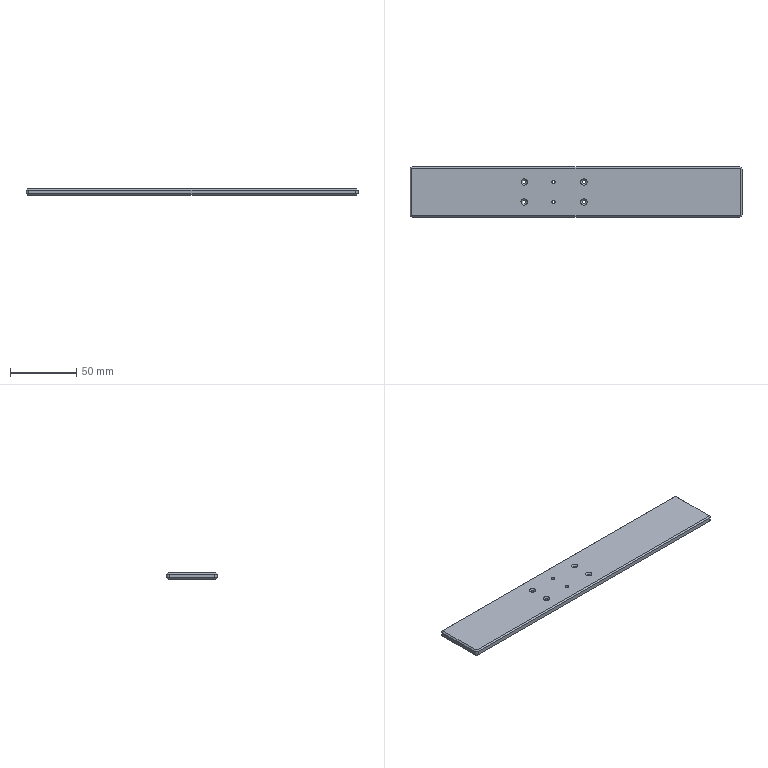CAM job | NX | 3-axis milling | part box 250 x 38 x 5 mm | stock box 256 x 44 x 5 mm
Tools:
number,name,description,diameter,corner_radius,flute_length,length,flutes
2,D10,Milling Tool-5 Parameters,10.0,0.0,50.0,75.0,2
8,D2,Milling Tool-5 Parameters,2.0,0.0,50.0,75.0,2
9,D6A45,Milling Tool-5 Parameters,6.0,0.0,3.0,3.0,2
6,D4,Milling Tool-5 Parameters,4.0,0.0,50.0,75.0,2
Operations:
program,operation,operation_type,tool,method,geometry_group,spindle_rpm,surface_speed,feed_per_tooth,feed_cut,feed_plunge,cut_length_mm,path_length_mm,cut_time_min,machine_time_min
PN_0001_BLANK_-_SUCTION_CUP,ZLEVEL_PROFILE,ZLevelMilling,D10,METHOD,A,6500.0,326.0,0.1538,2000.0,1000.0,3125.06,3186.76,1.586,1.592
PN_0001_BLANK_-_SUCTION_CUP,ZLEVEL_PROFILE_COPY_COPY_1_COPY_COPY_1_COPY,ZLevelMilling,D2,METHOD,A,7000.0,43.0,0.0714,1000.0,1000.0,1380.772,1838.533,1.381,1.427
PN_0001_BLANK_-_SUCTION_CUP,ZLEVEL_PROFILE_COPY_1_COPY_COPY_COPY_COPY_COPY_COPY,ZLevelMilling,D6A45,METHOD,A,7000.0,131.0,0.0714,1000.0,1000.0,582.053,646.053,0.5821,0.5885
PN_0001_BLANK_-_SUCTION_CUP,ZLEVEL_PROFILE_COPY_COPY_1_COPY,ZLevelMilling,D4,METHOD,A,6000.0,75.0,0.0833,1000.0,1000.0,590.581,657.281,0.5906,0.5973